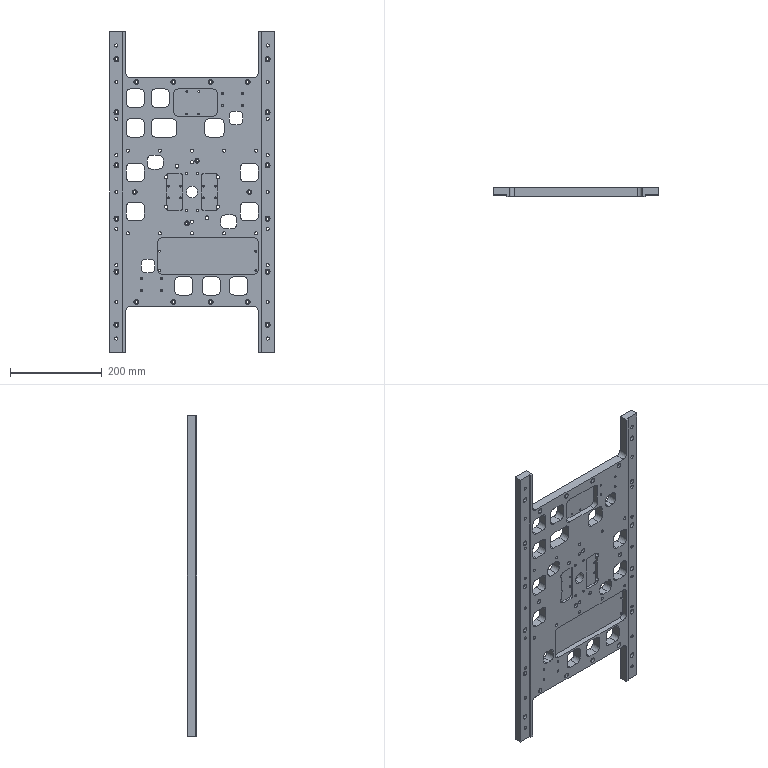Part | SolidWorks | features ICE 24, HoleWzd 12, RevCut 4, Fillet 2, Chamfer 1, Extrusion 1 | 1 solid | 517 faces | box 360 x 20 x 700 mm | volume 2898584 mm3 | cylinder 346 | plane 145 | cone 26 | commonest cylinder face diameters 20 x76 6.8 x68 6.6 x40 11 x40 5 x24 10 x24